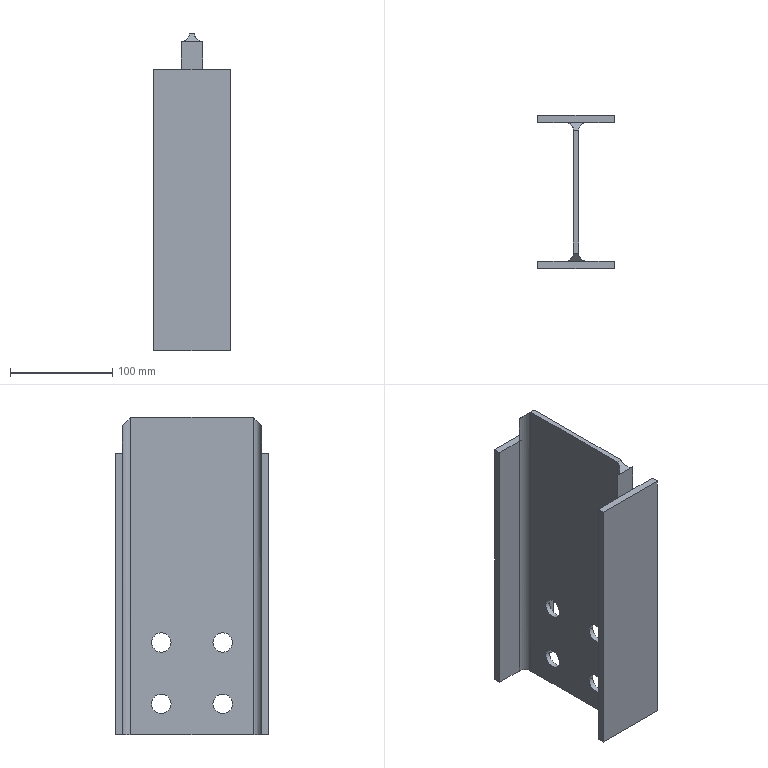Part | STEP file | 粉仓辅梁4主体_Default<As Machined> | 1 solid | 32 faces | box 75 x 150 x 310 mm | volume 510249 mm3 | plane 20 | cylinder 12 | commonest cylinder face diameters 19 x8 16 x4